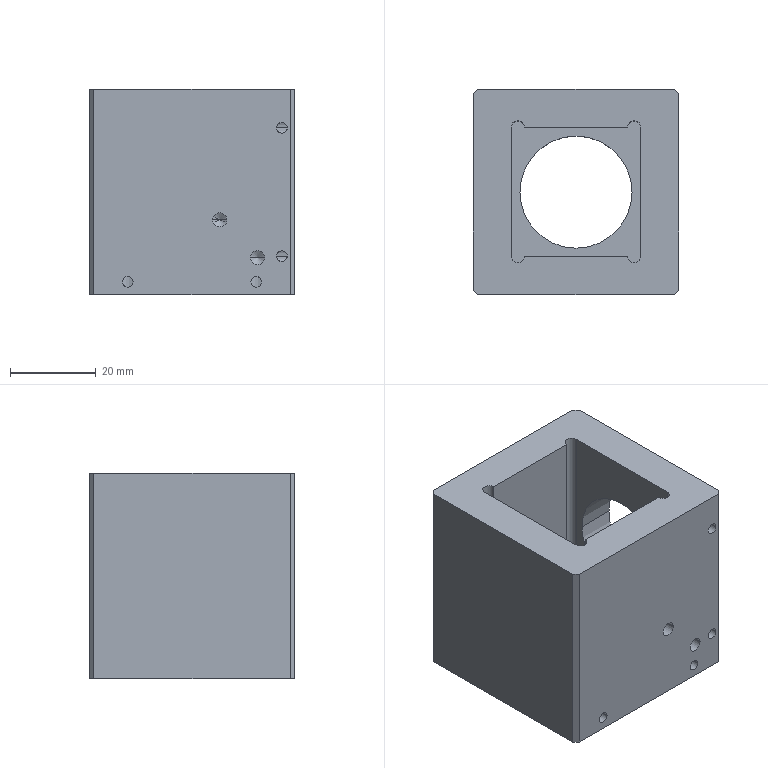NC program | NX | posted with a generic post | part box 48 x 48 x 48 mm
Whole program:
N10 G17 G21 G94 G90
(HOLE_MILLING_COPY , TOOL : D10)
N12 T15 M6
N14 G54
N16 G17 G0 G90 X0. Y0. B0. C0. S9500 M3
N18 G43 Z30. H15
N20 Z0.5
N22 G94 G3 X2. Y-2. R2. F2220.
N24 X4. Y0. R2.
N26 X4. Y0. Z-0.5 I-4. J0.
N28 X4. Y0. Z-1.5 I-4. J0.
N30 X4. Y0. Z-2.5 I-4. J0.
N32 X4. Y0. Z-3.5 I-4. J0.
N34 X4. Y0. Z-4.5 I-4. J0.
N36 X4. Y0. Z-5.5 I-4. J0.
N38 X4. Y0. Z-6.5 I-4. J0.
N40 X4. Y0. Z-7.5 I-4. J0.
N42 X4. Y0. Z-8.5 I-4. J0.
N44 X-3.236 Y2.351 Z-8.9 R4.
N46 X-2.351 Y-3.236 R4.
N48 X-3.236 Y2.351 R-4.
N50 X-2.794 Y-0.442 R2.
N52 X0. Y0. R2.
N54 G0 Z0.5
N56 G3 X4. Y-4. R4.
N58 X8. Y0. R4.
N60 X8. Y0. Z-0.5 I-8. J0.
N62 X8. Y0. Z-1.5 I-8. J0.
N64 X8. Y0. Z-2.5 I-8. J0.
N66 X8. Y0. Z-3.5 I-8. J0.
N68 X8. Y0. Z-4.5 I-8. J0.
N70 X8. Y0. Z-5.5 I-8. J0.
N72 X8. Y0. Z-6.5 I-8. J0.
N74 X8. Y0. Z-7.5 I-8. J0.
N76 X8. Y0. Z-8.5 I-8. J0.
N78 X-6.472 Y4.702 Z-8.9 R8.
N80 X-4.702 Y-6.472 R8.
N82 X-6.472 Y4.702 R-8.
N84 X-5.587 Y-0.885 R4.
N86 X0. Y0. R4.
N88 G0 Z30.
N90 M5
(ZLEVEL_PROFILE_COPY_1_COPY_COPY_1_COPY_COPY_COPY_COPY , TOOL : D10JING)
N92 T14 M6
N94 G54
N96 G17 G0 G90 X1.909 Y5.794 B0. C0. S9500 M3
N98 G43 Z30. H14
N100 Z-7.9
N102 G94 G1 Z-8.9 F1000.
N104 X0.866 Y7.6
N106 G3 X0. Y8.1 R1.
N108 X-8.1 Y0. R8.1 F1200.
N110 X0. Y8.1 R-8.1
N112 X-0.866 Y7.6 R1.
N114 G1 X-1.909 Y5.794
N116 Z-7.9
N118 G0 Z30.
N120 M5
(HOLE_MILLING_1_COPY , TOOL : D4)
N122 T11 M6
N124 G54
N126 G17 G0 G90 X-15. Y15. B0. C0. S9500 M3
N128 G43 Z30. H11
N130 Z0.5
N132 G94 G3 X-14.55 Y14.55 R0.45 F1650.
N134 X-14.1 Y15. R0.45
N136 X-14.1 Y15. Z0.1 I-0.9 J0.
N138 X-14.1 Y15. Z-0.3 I-0.9 J0.
N140 X-14.1 Y15. Z-0.7 I-0.9 J0.
N142 X-14.1 Y15. Z-1.1 I-0.9 J0.
N144 X-14.1 Y15. Z-1.5 I-0.9 J0.
N146 X-14.1 Y15. Z-1.9 I-0.9 J0.
N148 X-14.1 Y15. Z-2.3 I-0.9 J0.
N150 X-14.1 Y15. Z-2.7 I-0.9 J0.
N152 X-14.1 Y15. Z-3.1 I-0.9 J0.
N154 X-14.1 Y15. Z-3.5 I-0.9 J0.
N156 X-14.1 Y15. Z-3.9 I-0.9 J0.
N158 X-14.1 Y15. Z-4.3 I-0.9 J0.
N160 X-14.1 Y15. Z-4.7 I-0.9 J0.
N162 X-14.1 Y15. Z-5.1 I-0.9 J0.
N164 X-14.1 Y15. Z-5.5 I-0.9 J0.
N166 X-15. Y14.1 Z-5.8 R-0.9
N168 X-14.1 Y15. R0.9
N170 X-15. Y14.1 R-0.9
N172 X-14.55 Y14.55 R0.45
N174 X-15. Y15. R0.45
N176 G0 Z30.
N178 Y-15.
N180 Z0.5
N182 G3 X-14.55 Y-15.45 R0.45
N184 X-14.1 Y-15. R0.45
N186 X-14.1 Y-15. Z0.1 I-0.9 J0.
N188 X-14.1 Y-15. Z-0.3 I-0.9 J0.
N190 X-14.1 Y-15. Z-0.7 I-0.9 J0.
N192 X-14.1 Y-15. Z-1.1 I-0.9 J0.
N194 X-14.1 Y-15. Z-1.5 I-0.9 J0.
N196 X-14.1 Y-15. Z-1.9 I-0.9 J0.
N198 X-14.1 Y-15. Z-2.3 I-0.9 J0.
N200 X-14.1 Y-15. Z-2.7 I-0.9 J0.
N202 X-14.1 Y-15. Z-3.1 I-0.9 J0.
N204 X-14.1 Y-15. Z-3.5 I-0.9 J0.
N206 X-14.1 Y-15. Z-3.9 I-0.9 J0.
N208 X-14.1 Y-15. Z-4.3 I-0.9 J0.
N210 X-14.1 Y-15. Z-4.7 I-0.9 J0.
N212 X-14.1 Y-15. Z-5.1 I-0.9 J0.
N214 X-14.1 Y-15. Z-5.5 I-0.9 J0.
N216 X-15. Y-15.9 Z-5.8 R-0.9
N218 X-14.1 Y-15. R0.9
N220 X-15. Y-15.9 R-0.9
N222 X-14.55 Y-15.45 R0.45
N224 X-15. Y-15. R0.45
N226 G0 Z30.
N228 X15.
N230 Z0.5
N232 G3 X15.45 Y-15.45 R0.45
N234 X15.9 Y-15. R0.45
N236 X15.9 Y-15. Z0.1 I-0.9 J0.
N238 X15.9 Y-15. Z-0.3 I-0.9 J0.
N240 X15.9 Y-15. Z-0.7 I-0.9 J0.
N242 X15.9 Y-15. Z-1.1 I-0.9 J0.
N244 X15.9 Y-15. Z-1.5 I-0.9 J0.
N246 X15.9 Y-15. Z-1.9 I-0.9 J0.
N248 X15.9 Y-15. Z-2.3 I-0.9 J0.
N250 X15.9 Y-15. Z-2.7 I-0.9 J0.
N252 X15.9 Y-15. Z-3.1 I-0.9 J0.
N254 X15.9 Y-15. Z-3.5 I-0.9 J0.
N256 X15.9 Y-15. Z-3.9 I-0.9 J0.
N258 X15.9 Y-15. Z-4.3 I-0.9 J0.
N260 X15.9 Y-15. Z-4.7 I-0.9 J0.
N262 X15.9 Y-15. Z-5.1 I-0.9 J0.
N264 X15.9 Y-15. Z-5.5 I-0.9 J0.
N266 X15. Y-15.9 Z-5.8 R-0.9
N268 X15.9 Y-15. R0.9
N270 X15. Y-15.9 R-0.9
N272 X15.45 Y-15.45 R0.45
N274 X15. Y-15. R0.45
N276 G0 Z30.
N278 Y15.
N280 Z0.5
N282 G3 X15.45 Y14.55 R0.45
N284 X15.9 Y15. R0.45
N286 X15.9 Y15. Z0.1 I-0.9 J0.
N288 X15.9 Y15. Z-0.3 I-0.9 J0.
N290 X15.9 Y15. Z-0.7 I-0.9 J0.
N292 X15.9 Y15. Z-1.1 I-0.9 J0.
N294 X15.9 Y15. Z-1.5 I-0.9 J0.
N296 X15.9 Y15. Z-1.9 I-0.9 J0.
N298 X15.9 Y15. Z-2.3 I-0.9 J0.
N300 X15.9 Y15. Z-2.7 I-0.9 J0.
N302 X15.9 Y15. Z-3.1 I-0.9 J0.
N304 X15.9 Y15. Z-3.5 I-0.9 J0.
N306 X15.9 Y15. Z-3.9 I-0.9 J0.
N308 X15.9 Y15. Z-4.3 I-0.9 J0.
N310 X15.9 Y15. Z-4.7 I-0.9 J0.
N312 X15.9 Y15. Z-5.1 I-0.9 J0.
N314 X15.9 Y15. Z-5.5 I-0.9 J0.
N316 X15. Y14.1 Z-5.8 R-0.9
N318 X15.9 Y15. R0.9
N320 X15. Y14.1 R-0.9
N322 X15.45 Y14.55 R0.45
N324 X15. Y15. R0.45
N326 G0 Z30.
N328 M5
(PLANAR_MILL_COPY_COPY_COPY_COPY_COPY_COPY_1_COPY_1_COPY_COPY , TOOL : D6A45)
N330 T01 M6
N332 G54
N334 G17 G0 G90 X15.891 Y-15.454 B0. C0. S9500 M3
N336 G43 Z30. H1
N338 Z0.5
N340 G94 G1 Z-1. F1250.
N342 X16.7 Y-15.866
N344 G3 X17.2 Y-15. R1.
N346 X15. Y-12.8 R2.2
N348 X17.2 Y-15. R-2.2
N350 X16.7 Y-14.134 R1.
N352 G1 X15.891 Y-14.546
N354 Z0.5
N356 G0 Z30.
N358 Y14.546
N360 Z0.5
N362 G1 Z-1.
N364 X16.7 Y14.134
N366 G3 X17.2 Y15. R1.
N368 X15. Y17.2 R2.2
N370 X17.2 Y15. R-2.2
N372 X16.7 Y15.866 R1.
N374 G1 X15.891 Y15.454
N376 Z0.5
N378 G0 Z30.
N380 X-15.891
N382 Z0.5
N384 G1 Z-1.
N386 X-16.7 Y15.866
N388 G3 X-17.2 Y15. R1.
N390 X-15. Y12.8 R2.2
N392 X-17.2 Y15. R-2.2
N394 X-16.7 Y14.134 R1.
N396 G1 X-15.891 Y14.546
N398 Z0.5
N400 G0 Z30.
N402 X-11.022 Y1.315
N404 Z0.5
N406 G1 Z-1.
N408 X-11.8 Y0.866
N410 G3 X-12.3 Y0. R1.
N412 X0. Y-12.3 R12.3
N414 X-12.3 Y0. R-12.3
N416 X-11.8 Y-0.866 R1.
N418 G1 X-11.022 Y-1.315
N420 Z0.5
N422 G0 Z30.
N424 X-15.891 Y-14.546
N426 Z0.5
N428 G1 Z-1.
N430 X-16.7 Y-14.134
N432 G3 X-17.2 Y-15. R1.
N434 X-15. Y-17.2 R2.2
N436 X-17.2 Y-15. R-2.2
N438 X-16.7 Y-15.866 R1.
N440 G1 X-15.891 Y-15.454
N442 Z0.5
N444 G0 Z30.
N446 M5
(刀补11_COPY , TOOL : D4)
N448 T11 M6
N450 G54
N452 G17 G0 G90 X-15. Y15. B0. C0. S9500 M3
N454 G43 Z30. H11
N456 Z0.5
N458 G41 G94 G1 X-14.996 Y14.9 F1000. D11
N460 G3 X-14.05 Y15. R0.478
N462 X-14.05 Y15. Z-1.5 I-0.95 J0.
N464 X-14.05 Y15. Z-3.5 I-0.95 J0.
N466 X-14.05 Y15. Z-5.5 I-0.95 J0.
N468 X-14.442 Y15.769 Z-5.8 R0.95
N470 X-15.769 Y15.558 R0.95
N472 X-14.442 Y15.769 R-0.95
N474 X-15.079 Y15.062 R0.478
N476 G40
N478 G1 X-15. Y15.
N480 G0 Z30.
N482 Y-15.
N484 Z0.5
N486 G41 G1 X-14.996 Y-15.1
N488 G3 X-14.05 Y-15. R0.478
N490 X-14.05 Y-15. Z-1.5 I-0.95 J0.
N492 X-14.05 Y-15. Z-3.5 I-0.95 J0.
N494 X-14.05 Y-15. Z-5.5 I-0.95 J0.
N496 X-14.442 Y-14.231 Z-5.8 R0.95
N498 X-15.769 Y-14.442 R0.95
N500 X-14.442 Y-14.231 R-0.95
N502 X-15.079 Y-14.938 R0.478
N504 G40
N506 G1 X-15. Y-15.
N508 G0 Z30.
N510 X15.
N512 Z0.5
N514 G41 G1 X15.004 Y-15.1
N516 G3 X15.95 Y-15. R0.478
N518 X15.95 Y-15. Z-1.5 I-0.95 J0.
N520 X15.95 Y-15. Z-3.5 I-0.95 J0.
N522 X15.95 Y-15. Z-5.5 I-0.95 J0.
N524 X15.558 Y-14.231 Z-5.8 R0.95
N526 X14.231 Y-14.442 R0.95
N528 X15.558 Y-14.231 R-0.95
N530 X14.921 Y-14.938 R0.478
N532 G40
N534 G1 X15. Y-15.
N536 G0 Z30.
N538 Y15.
N540 Z0.5
N542 G41 G1 X15.004 Y14.9
N544 G3 X15.95 Y15. R0.478
N546 X15.95 Y15. Z-1.5 I-0.95 J0.
N548 X15.95 Y15. Z-3.5 I-0.95 J0.
N550 X15.95 Y15. Z-5.5 I-0.95 J0.
N552 X15.558 Y15.769 Z-5.8 R0.95
N554 X14.231 Y15.558 R0.95
N556 X15.558 Y15.769 R-0.95
N558 X14.921 Y15.062 R0.478
N560 G40
N562 G1 X15. Y15.
N564 G0 Z30.
N566 M5
N568 M2